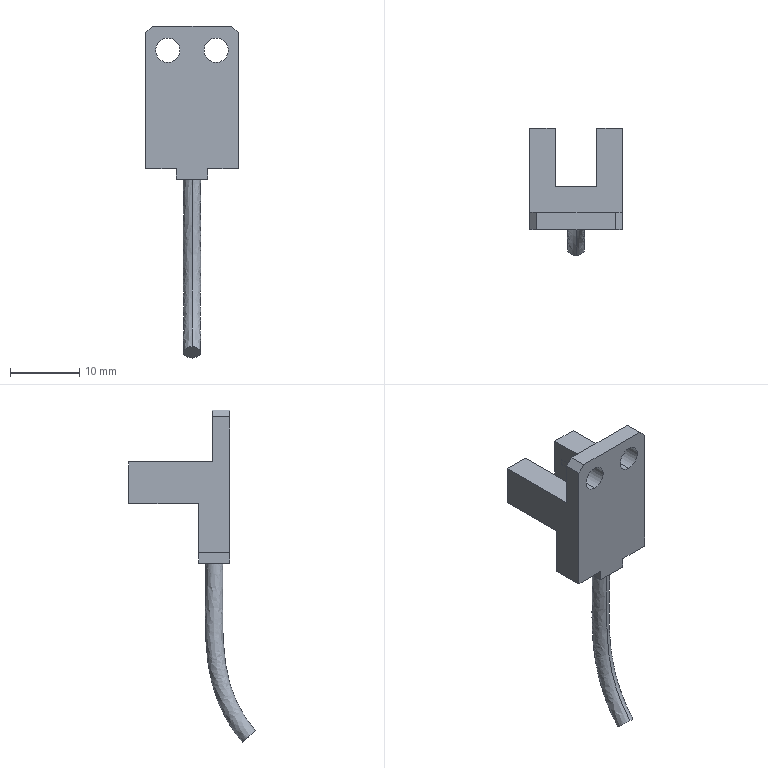Part | NX | features BREP 1 | 1 solid | 41 faces | box 13.4 x 18.3 x 47.912 mm | volume 1659 mm3 | plane 33 | cylinder 6 | spline 2 | commonest cylinder face diameters 3.5 x4 1 x2
STEP:
#1=CARTESIAN_POINT('',(1.25,2.25,-8.6));
#2=VERTEX_POINT('',#1);
#3=CARTESIAN_POINT('',(0.,0.9995,-8.6));
#4=VERTEX_POINT('',#3);
#5=CARTESIAN_POINT('',(1.25,2.25,-8.6));
#6=CARTESIAN_POINT('',(1.25,1.59,-8.6));
#7=CARTESIAN_POINT('',(0.6604,0.9995,-8.6));
#8=CARTESIAN_POINT('',(0.,0.9995,-8.6));
#9=B_SPLINE_CURVE_WITH_KNOTS('',3,(#5,#6,#7,#8),.UNSPECIFIED.,.F.,.F.,(4,4),(0.,0.001953),.UNSPECIFIED.);
#10=EDGE_CURVE('',#2,#4,#9,.T.);
#11=ORIENTED_EDGE('',*,*,#10,.T.);
#12=CARTESIAN_POINT('',(0.,-3.7,-32.788));
#13=VERTEX_POINT('',#12);
#14=CARTESIAN_POINT('',(0.,0.9995,-8.6));
#15=CARTESIAN_POINT('',(0.,0.8731,-12.965));
#16=CARTESIAN_POINT('',(0.,1.227,-17.286));
#17=CARTESIAN_POINT('',(0.,0.4346,-25.439));
#18=CARTESIAN_POINT('',(0.,-0.6656,-29.235));
#19=CARTESIAN_POINT('',(0.,-3.7,-32.788));
#20=B_SPLINE_CURVE_WITH_KNOTS('',3,(#14,#15,#16,#17,#18,#19),.UNSPECIFIED.,.F.,.F.,(4,2,4),(0.,0.4993,1.),.UNSPECIFIED.);
#21=EDGE_CURVE('',#4,#13,#20,.T.);
#22=ORIENTED_EDGE('',*,*,#21,.T.);
#23=CARTESIAN_POINT('',(0.,-1.8,-34.412));
#24=VERTEX_POINT('',#23);
#25=CARTESIAN_POINT('',(0.,-2.75,-33.6));
#26=DIRECTION('',(0.,-0.6495,-0.7604));
#27=DIRECTION('',(0.,0.7604,-0.6495));
#28=AXIS2_PLACEMENT_3D('',#25,#26,#27);
#29=CIRCLE('',#28,1.25);
#30=EDGE_CURVE('',#24,#13,#29,.T.);
#31=ORIENTED_EDGE('',*,*,#30,.F.);
#32=CARTESIAN_POINT('',(0.,3.499,-8.637));
#33=VERTEX_POINT('',#32);
#34=CARTESIAN_POINT('',(0.,3.499,-8.637));
#35=CARTESIAN_POINT('',(0.,3.376,-12.823));
#36=CARTESIAN_POINT('',(0.,3.746,-17.21));
#37=CARTESIAN_POINT('',(0.,2.893,-25.986));
#38=CARTESIAN_POINT('',(0.,1.62,-30.408));
#39=CARTESIAN_POINT('',(0.,-1.8,-34.412));
#40=B_SPLINE_CURVE_WITH_KNOTS('',3,(#34,#35,#36,#37,#38,#39),.UNSPECIFIED.,.F.,.F.,(4,2,4),(0.,0.5,1.),.UNSPECIFIED.);
#41=EDGE_CURVE('',#33,#24,#40,.T.);
#42=ORIENTED_EDGE('',*,*,#41,.F.);
#43=CARTESIAN_POINT('',(0.,2.25,-8.6));
#44=DIRECTION('',(0.,-0.02956,-0.9996));
#45=DIRECTION('',(0.,0.9996,-0.02956));
#46=AXIS2_PLACEMENT_3D('',#43,#44,#45);
#47=CIRCLE('',#46,1.25);
#48=EDGE_CURVE('',#33,#2,#47,.T.);
#49=ORIENTED_EDGE('',*,*,#48,.T.);
#50=EDGE_LOOP('',(#11,#22,#31,#42,#49));
#51=FACE_BOUND('',#50,.T.);
#52=CARTESIAN_POINT('',(0.,3.499,-8.637));
#53=CARTESIAN_POINT('',(0.,3.376,-12.823));
#54=CARTESIAN_POINT('',(0.,3.746,-17.21));
#55=CARTESIAN_POINT('',(0.,2.893,-25.986));
#56=CARTESIAN_POINT('',(0.,1.62,-30.408));
#57=CARTESIAN_POINT('',(0.,-1.8,-34.412));
#58=CARTESIAN_POINT('',(2.5,3.499,-8.637));
#59=CARTESIAN_POINT('',(2.5,3.376,-12.823));
#60=CARTESIAN_POINT('',(2.5,3.746,-17.21));
#61=CARTESIAN_POINT('',(2.5,2.893,-25.986));
#62=CARTESIAN_POINT('',(2.5,1.62,-30.408));
#63=CARTESIAN_POINT('',(2.5,-1.8,-34.412));
#64=CARTESIAN_POINT('',(2.5,1.001,-8.563));
#65=CARTESIAN_POINT('',(2.5,0.8711,-12.94));
#66=CARTESIAN_POINT('',(2.5,1.228,-17.274));
#67=CARTESIAN_POINT('',(2.5,0.4346,-25.439));
#68=CARTESIAN_POINT('',(2.5,-0.6656,-29.235));
#69=CARTESIAN_POINT('',(2.5,-3.7,-32.788));
#70=CARTESIAN_POINT('',(0.,1.001,-8.563));
#71=CARTESIAN_POINT('',(0.,0.8711,-12.94));
#72=CARTESIAN_POINT('',(0.,1.228,-17.274));
#73=CARTESIAN_POINT('',(0.,0.4346,-25.439));
#74=CARTESIAN_POINT('',(0.,-0.6656,-29.235));
#75=CARTESIAN_POINT('',(0.,-3.7,-32.788));
#76=(BOUNDED_SURFACE()B_SPLINE_SURFACE(3,3,((#52,#53,#54,#55,#56,#57),(#58,#59,#60,#61,#62,#63),(#64,#65,#66,#67,#68,#69),(#70,#71,#72,#73,#74,#75)),.UNSPECIFIED.,.F.,.F.,.F.)B_SPLINE_SURFACE_WITH_KNOTS((4,4),(4,2,4),(0.,0.5),(0.,0.5,1.),.UNSPECIFIED.)GEOMETRIC_REPRESENTATION_ITEM()RATIONAL_B_SPLINE_SURFACE(((1.,1.,1.,1.,1.,1.),(0.3333,0.3333,0.3333,0.3333,0.3333,0.3333),(0.3333,0.3333,0.3333,0.3333,0.3333,0.3333),(1.,1.,1.,1.,1.,1.)))REPRESENTATION_ITEM('')SURFACE());
#77=ADVANCED_FACE('',(#51),#76,.T.);
#78=CARTESIAN_POINT('',(3.502,2.5,11.75));
#79=VERTEX_POINT('',#78);
#80=CARTESIAN_POINT('',(3.502,2.5,8.25));
#81=VERTEX_POINT('',#80);
#82=CARTESIAN_POINT('',(3.502,2.5,10.));
#83=DIRECTION('',(0.,-1.,0.));
#84=DIRECTION('',(0.,0.,-1.));
#85=AXIS2_PLACEMENT_3D('',#82,#83,#84);
#86=CIRCLE('',#85,1.75);
#87=EDGE_CURVE('',#79,#81,#86,.T.);
#88=ORIENTED_EDGE('',*,*,#87,.F.);
#89=CARTESIAN_POINT('',(3.502,0.,11.75));
#90=VERTEX_POINT('',#89);
#91=CARTESIAN_POINT('',(3.502,14.6,11.75));
#92=DIRECTION('',(0.,-1.,0.));
#93=VECTOR('',#92,1000.);
#94=LINE('',#91,#93);
#95=EDGE_CURVE('',#90,#79,#94,.F.);
#96=ORIENTED_EDGE('',*,*,#95,.F.);
#97=CARTESIAN_POINT('',(3.502,0.,8.25));
#98=VERTEX_POINT('',#97);
#99=CARTESIAN_POINT('',(3.502,0.,10.));
#100=DIRECTION('',(0.,1.,0.));
#101=DIRECTION('',(0.,0.,1.));
#102=AXIS2_PLACEMENT_3D('',#99,#100,#101);
#103=CIRCLE('',#102,1.75);
#104=EDGE_CURVE('',#98,#90,#103,.T.);
#105=ORIENTED_EDGE('',*,*,#104,.F.);
#106=CARTESIAN_POINT('',(3.502,14.6,8.25));
#107=DIRECTION('',(0.,-1.,0.));
#108=VECTOR('',#107,1000.);
#109=LINE('',#106,#108);
#110=EDGE_CURVE('',#98,#81,#109,.F.);
#111=ORIENTED_EDGE('',*,*,#110,.T.);
#112=EDGE_LOOP('',(#88,#96,#105,#111));
#113=FACE_BOUND('',#112,.T.);
#114=CARTESIAN_POINT('',(3.502,14.6,10.));
#115=DIRECTION('',(0.,-1.,0.));
#116=DIRECTION('',(0.,0.,1.));
#117=AXIS2_PLACEMENT_3D('',#114,#115,#116);
#118=CYLINDRICAL_SURFACE('',#117,1.75);
#119=ADVANCED_FACE('',(#113),#118,.F.);
#120=CARTESIAN_POINT('',(-3.502,2.5,11.75));
#121=VERTEX_POINT('',#120);
#122=CARTESIAN_POINT('',(-3.502,2.5,8.25));
#123=VERTEX_POINT('',#122);
#124=CARTESIAN_POINT('',(-3.502,2.5,10.));
#125=DIRECTION('',(0.,-1.,0.));
#126=DIRECTION('',(0.,0.,-1.));
#127=AXIS2_PLACEMENT_3D('',#124,#125,#126);
#128=CIRCLE('',#127,1.75);
#129=EDGE_CURVE('',#121,#123,#128,.T.);
#130=ORIENTED_EDGE('',*,*,#129,.F.);
#131=CARTESIAN_POINT('',(-3.502,0.,11.75));
#132=VERTEX_POINT('',#131);
#133=CARTESIAN_POINT('',(-3.502,14.6,11.75));
#134=DIRECTION('',(0.,-1.,0.));
#135=VECTOR('',#134,1000.);
#136=LINE('',#133,#135);
#137=EDGE_CURVE('',#132,#121,#136,.F.);
#138=ORIENTED_EDGE('',*,*,#137,.F.);
#139=CARTESIAN_POINT('',(-3.502,0.,8.25));
#140=VERTEX_POINT('',#139);
#141=CARTESIAN_POINT('',(-3.502,0.,10.));
#142=DIRECTION('',(0.,1.,0.));
#143=DIRECTION('',(0.,0.,1.));
#144=AXIS2_PLACEMENT_3D('',#141,#142,#143);
#145=CIRCLE('',#144,1.75);
#146=EDGE_CURVE('',#140,#132,#145,.T.);
#147=ORIENTED_EDGE('',*,*,#146,.F.);
#148=CARTESIAN_POINT('',(-3.502,14.6,8.25));
#149=DIRECTION('',(0.,-1.,0.));
#150=VECTOR('',#149,1000.);
#151=LINE('',#148,#150);
#152=EDGE_CURVE('',#140,#123,#151,.F.);
#153=ORIENTED_EDGE('',*,*,#152,.T.);
#154=EDGE_LOOP('',(#130,#138,#147,#153));
#155=FACE_BOUND('',#154,.T.);
#156=CARTESIAN_POINT('',(-3.502,14.6,10.));
#157=DIRECTION('',(0.,-1.,0.));
#158=DIRECTION('',(0.,0.,1.));
#159=AXIS2_PLACEMENT_3D('',#156,#157,#158);
#160=CYLINDRICAL_SURFACE('',#159,1.75);
#161=ADVANCED_FACE('',(#155),#160,.F.);
#162=CARTESIAN_POINT('',(0.,6.21,3.5));
#163=VERTEX_POINT('',#162);
#164=CARTESIAN_POINT('',(0.,6.21,2.5));
#165=VERTEX_POINT('',#164);
#166=CARTESIAN_POINT('',(0.,6.21,3.));
#167=DIRECTION('',(0.,1.,0.));
#168=DIRECTION('',(0.,0.,1.));
#169=AXIS2_PLACEMENT_3D('',#166,#167,#168);
#170=CIRCLE('',#169,0.5);
#171=EDGE_CURVE('',#163,#165,#170,.T.);
#172=ORIENTED_EDGE('',*,*,#171,.F.);
#173=CARTESIAN_POINT('',(0.,6.2,3.5));
#174=VERTEX_POINT('',#173);
#175=CARTESIAN_POINT('',(0.,6.21,3.5));
#176=DIRECTION('',(0.,-1.,0.));
#177=VECTOR('',#176,1000.);
#178=LINE('',#175,#177);
#179=EDGE_CURVE('',#174,#163,#178,.F.);
#180=ORIENTED_EDGE('',*,*,#179,.F.);
#181=CARTESIAN_POINT('',(0.,6.2,2.5));
#182=VERTEX_POINT('',#181);
#183=CARTESIAN_POINT('',(0.,6.2,3.));
#184=DIRECTION('',(0.,1.,0.));
#185=DIRECTION('',(0.,0.,-1.));
#186=AXIS2_PLACEMENT_3D('',#183,#184,#185);
#187=CIRCLE('',#186,0.5);
#188=EDGE_CURVE('',#174,#182,#187,.T.);
#189=ORIENTED_EDGE('',*,*,#188,.T.);
#190=CARTESIAN_POINT('',(0.,6.21,2.5));
#191=DIRECTION('',(0.,-1.,0.));
#192=VECTOR('',#191,1000.);
#193=LINE('',#190,#192);
#194=EDGE_CURVE('',#182,#165,#193,.F.);
#195=ORIENTED_EDGE('',*,*,#194,.T.);
#196=EDGE_LOOP('',(#172,#180,#189,#195));
#197=FACE_BOUND('',#196,.T.);
#198=CARTESIAN_POINT('',(0.,6.21,3.));
#199=DIRECTION('',(0.,-1.,0.));
#200=DIRECTION('',(0.,0.,1.));
#201=AXIS2_PLACEMENT_3D('',#198,#199,#200);
#202=CYLINDRICAL_SURFACE('',#201,0.5);
#203=ADVANCED_FACE('',(#197),#202,.T.);
#204=CARTESIAN_POINT('',(2.25,4.5,-8.6));
#205=VERTEX_POINT('',#204);
#206=CARTESIAN_POINT('',(2.25,0.,-8.6));
#207=VERTEX_POINT('',#206);
#208=CARTESIAN_POINT('',(2.25,4.5,-8.6));
#209=DIRECTION('',(0.,-1.,0.));
#210=VECTOR('',#209,1000.);
#211=LINE('',#208,#210);
#212=EDGE_CURVE('',#205,#207,#211,.T.);
#213=ORIENTED_EDGE('',*,*,#212,.T.);
#214=CARTESIAN_POINT('',(-2.25,0.,-8.6));
#215=VERTEX_POINT('',#214);
#216=CARTESIAN_POINT('',(2.25,0.,-8.6));
#217=DIRECTION('',(-1.,0.,0.));
#218=VECTOR('',#217,1000.);
#219=LINE('',#216,#218);
#220=EDGE_CURVE('',#207,#215,#219,.T.);
#221=ORIENTED_EDGE('',*,*,#220,.T.);
#222=CARTESIAN_POINT('',(-2.25,4.5,-8.6));
#223=VERTEX_POINT('',#222);
#224=CARTESIAN_POINT('',(-2.25,4.5,-8.6));
#225=DIRECTION('',(0.,1.,0.));
#226=VECTOR('',#225,1000.);
#227=LINE('',#224,#226);
#228=EDGE_CURVE('',#215,#223,#227,.T.);
#229=ORIENTED_EDGE('',*,*,#228,.T.);
#230=CARTESIAN_POINT('',(2.25,4.5,-8.6));
#231=DIRECTION('',(1.,0.,0.));
#232=VECTOR('',#231,1000.);
#233=LINE('',#230,#232);
#234=EDGE_CURVE('',#223,#205,#233,.T.);
#235=ORIENTED_EDGE('',*,*,#234,.T.);
#236=EDGE_LOOP('',(#213,#221,#229,#235));
#237=FACE_BOUND('',#236,.T.);
#238=ORIENTED_EDGE('',*,*,#10,.F.);
#239=CARTESIAN_POINT('',(-1.25,2.25,-8.6));
#240=VERTEX_POINT('',#239);
#241=CARTESIAN_POINT('',(0.,2.25,-8.6));
#242=DIRECTION('',(-1.,0.,0.));
#243=VECTOR('',#242,1000.);
#244=LINE('',#241,#243);
#245=EDGE_CURVE('',#2,#240,#244,.T.);
#246=ORIENTED_EDGE('',*,*,#245,.T.);
#247=CARTESIAN_POINT('',(0.,0.9995,-8.6));
#248=CARTESIAN_POINT('',(-0.6604,0.9995,-8.6));
#249=CARTESIAN_POINT('',(-1.25,1.59,-8.6));
#250=CARTESIAN_POINT('',(-1.25,2.25,-8.6));
#251=B_SPLINE_CURVE_WITH_KNOTS('',3,(#247,#248,#249,#250),.UNSPECIFIED.,.F.,.F.,(4,4),(0.,0.001953),.UNSPECIFIED.);
#252=EDGE_CURVE('',#4,#240,#251,.T.);
#253=ORIENTED_EDGE('',*,*,#252,.F.);
#254=EDGE_LOOP('',(#238,#246,#253));
#255=FACE_BOUND('',#254,.T.);
#256=CARTESIAN_POINT('',(0.,0.,-8.6));
#257=DIRECTION('',(0.,0.,-1.));
#258=DIRECTION('',(1.,0.,0.));
#259=AXIS2_PLACEMENT_3D('',#256,#257,#258);
#260=PLANE('',#259);
#261=ADVANCED_FACE('',(#237,#255),#260,.T.);
#262=CARTESIAN_POINT('',(2.25,4.5,-7.1));
#263=VERTEX_POINT('',#262);
#264=CARTESIAN_POINT('',(2.25,0.,-7.1));
#265=VERTEX_POINT('',#264);
#266=CARTESIAN_POINT('',(2.25,4.5,-7.1));
#267=DIRECTION('',(0.,-1.,0.));
#268=VECTOR('',#267,1000.);
#269=LINE('',#266,#268);
#270=EDGE_CURVE('',#263,#265,#269,.T.);
#271=ORIENTED_EDGE('',*,*,#270,.F.);
#272=CARTESIAN_POINT('',(6.7,4.5,-7.1));
#273=VERTEX_POINT('',#272);
#274=CARTESIAN_POINT('',(-6.7,4.5,-7.1));
#275=DIRECTION('',(1.,0.,0.));
#276=VECTOR('',#275,1000.);
#277=LINE('',#274,#276);
#278=EDGE_CURVE('',#263,#273,#277,.T.);
#279=ORIENTED_EDGE('',*,*,#278,.T.);
#280=CARTESIAN_POINT('',(6.7,0.,-7.1));
#281=VERTEX_POINT('',#280);
#282=CARTESIAN_POINT('',(6.7,4.5,-7.1));
#283=DIRECTION('',(0.,-1.,0.));
#284=VECTOR('',#283,1000.);
#285=LINE('',#282,#284);
#286=EDGE_CURVE('',#273,#281,#285,.T.);
#287=ORIENTED_EDGE('',*,*,#286,.T.);
#288=CARTESIAN_POINT('',(-6.7,0.,-7.1));
#289=DIRECTION('',(1.,0.,0.));
#290=VECTOR('',#289,1000.);
#291=LINE('',#288,#290);
#292=EDGE_CURVE('',#265,#281,#291,.T.);
#293=ORIENTED_EDGE('',*,*,#292,.F.);
#294=EDGE_LOOP('',(#271,#279,#287,#293));
#295=FACE_BOUND('',#294,.T.);
#296=CARTESIAN_POINT('',(-6.7,4.5,-7.1));
#297=DIRECTION('',(0.,0.,-1.));
#298=DIRECTION('',(1.,0.,0.));
#299=AXIS2_PLACEMENT_3D('',#296,#297,#298);
#300=PLANE('',#299);
#301=ADVANCED_FACE('',(#295),#300,.T.);
#302=CARTESIAN_POINT('',(6.7,4.5,0.));
#303=VERTEX_POINT('',#302);
#304=CARTESIAN_POINT('',(6.7,14.6,0.));
#305=VERTEX_POINT('',#304);
#306=CARTESIAN_POINT('',(6.7,14.6,0.));
#307=DIRECTION('',(0.,1.,0.));
#308=VECTOR('',#307,1000.);
#309=LINE('',#306,#308);
#310=EDGE_CURVE('',#303,#305,#309,.T.);
#311=ORIENTED_EDGE('',*,*,#310,.F.);
#312=CARTESIAN_POINT('',(-6.7,4.5,0.));
#313=VERTEX_POINT('',#312);
#314=CARTESIAN_POINT('',(-6.7,4.5,0.));
#315=DIRECTION('',(-1.,0.,0.));
#316=VECTOR('',#315,1000.);
#317=LINE('',#314,#316);
#318=EDGE_CURVE('',#303,#313,#317,.T.);
#319=ORIENTED_EDGE('',*,*,#318,.T.);
#320=CARTESIAN_POINT('',(-6.7,14.6,0.));
#321=VERTEX_POINT('',#320);
#322=CARTESIAN_POINT('',(-6.7,14.6,0.));
#323=DIRECTION('',(0.,-1.,0.));
#324=VECTOR('',#323,1000.);
#325=LINE('',#322,#324);
#326=EDGE_CURVE('',#321,#313,#325,.T.);
#327=ORIENTED_EDGE('',*,*,#326,.F.);
#328=CARTESIAN_POINT('',(-3.,14.6,0.));
#329=VERTEX_POINT('',#328);
#330=CARTESIAN_POINT('',(-3.,14.6,0.));
#331=DIRECTION('',(-1.,0.,0.));
#332=VECTOR('',#331,1000.);
#333=LINE('',#330,#332);
#334=EDGE_CURVE('',#329,#321,#333,.T.);
#335=ORIENTED_EDGE('',*,*,#334,.F.);
#336=CARTESIAN_POINT('',(-3.,6.2,0.));
#337=VERTEX_POINT('',#336);
#338=CARTESIAN_POINT('',(-3.,6.2,0.));
#339=DIRECTION('',(0.,1.,0.));
#340=VECTOR('',#339,1000.);
#341=LINE('',#338,#340);
#342=EDGE_CURVE('',#337,#329,#341,.T.);
#343=ORIENTED_EDGE('',*,*,#342,.F.);
#344=CARTESIAN_POINT('',(3.,6.2,0.));
#345=VERTEX_POINT('',#344);
#346=CARTESIAN_POINT('',(3.,6.2,0.));
#347=DIRECTION('',(-1.,0.,0.));
#348=VECTOR('',#347,1000.);
#349=LINE('',#346,#348);
#350=EDGE_CURVE('',#345,#337,#349,.T.);
#351=ORIENTED_EDGE('',*,*,#350,.F.);
#352=CARTESIAN_POINT('',(3.,14.6,0.));
#353=VERTEX_POINT('',#352);
#354=CARTESIAN_POINT('',(3.,6.2,0.));
#355=DIRECTION('',(0.,-1.,0.));
#356=VECTOR('',#355,1000.);
#357=LINE('',#354,#356);
#358=EDGE_CURVE('',#353,#345,#357,.T.);
#359=ORIENTED_EDGE('',*,*,#358,.F.);
#360=CARTESIAN_POINT('',(3.,14.6,0.));
#361=DIRECTION('',(-1.,0.,0.));
#362=VECTOR('',#361,1000.);
#363=LINE('',#360,#362);
#364=EDGE_CURVE('',#305,#353,#363,.T.);
#365=ORIENTED_EDGE('',*,*,#364,.F.);
#366=EDGE_LOOP('',(#311,#319,#327,#335,#343,#351,#359,#365));
#367=FACE_BOUND('',#366,.T.);
#368=CARTESIAN_POINT('',(0.,0.,0.));
#369=DIRECTION('',(0.,0.,-1.));
#370=DIRECTION('',(1.,0.,0.));
#371=AXIS2_PLACEMENT_3D('',#368,#369,#370);
#372=PLANE('',#371);
#373=ADVANCED_FACE('',(#367),#372,.T.);
#374=ORIENTED_EDGE('',*,*,#342,.T.);
#375=CARTESIAN_POINT('',(-3.,14.6,6.));
#376=VERTEX_POINT('',#375);
#377=CARTESIAN_POINT('',(-3.,14.6,6.));
#378=DIRECTION('',(0.,0.,-1.));
#379=VECTOR('',#378,1000.);
#380=LINE('',#377,#379);
#381=EDGE_CURVE('',#376,#329,#380,.T.);
#382=ORIENTED_EDGE('',*,*,#381,.F.);
#383=CARTESIAN_POINT('',(-3.,6.2,6.));
#384=VERTEX_POINT('',#383);
#385=CARTESIAN_POINT('',(-3.,6.2,6.));
#386=DIRECTION('',(0.,1.,0.));
#387=VECTOR('',#386,1000.);
#388=LINE('',#385,#387);
#389=EDGE_CURVE('',#384,#376,#388,.T.);
#390=ORIENTED_EDGE('',*,*,#389,.F.);
#391=CARTESIAN_POINT('',(-3.,6.2,6.));
#392=DIRECTION('',(0.,0.,-1.));
#393=VECTOR('',#392,1000.);
#394=LINE('',#391,#393);
#395=EDGE_CURVE('',#384,#337,#394,.T.);
#396=ORIENTED_EDGE('',*,*,#395,.T.);
#397=EDGE_LOOP('',(#374,#382,#390,#396));
#398=FACE_BOUND('',#397,.T.);
#399=CARTESIAN_POINT('',(-3.,12.,2.6));
#400=VERTEX_POINT('',#399);
#401=CARTESIAN_POINT('',(-3.,13.2,2.6));
#402=VERTEX_POINT('',#401);
#403=CARTESIAN_POINT('',(-3.,13.2,2.6));
#404=DIRECTION('',(0.,1.,0.));
#405=VECTOR('',#404,1000.);
#406=LINE('',#403,#405);
#407=EDGE_CURVE('',#400,#402,#406,.T.);
#408=ORIENTED_EDGE('',*,*,#407,.F.);
#409=CARTESIAN_POINT('',(-3.,12.,3.4));
#410=VERTEX_POINT('',#409);
#411=CARTESIAN_POINT('',(-3.,12.,3.4));
#412=DIRECTION('',(0.,0.,-1.));
#413=VECTOR('',#412,1000.);
#414=LINE('',#411,#413);
#415=EDGE_CURVE('',#410,#400,#414,.T.);
#416=ORIENTED_EDGE('',*,*,#415,.F.);
#417=CARTESIAN_POINT('',(-3.,13.2,3.4));
#418=VERTEX_POINT('',#417);
#419=CARTESIAN_POINT('',(-3.,13.2,3.4));
#420=DIRECTION('',(0.,-1.,0.));
#421=VECTOR('',#420,1000.);
#422=LINE('',#419,#421);
#423=EDGE_CURVE('',#418,#410,#422,.T.);
#424=ORIENTED_EDGE('',*,*,#423,.F.);
#425=CARTESIAN_POINT('',(-3.,13.2,3.4));
#426=DIRECTION('',(0.,0.,1.));
#427=VECTOR('',#426,1000.);
#428=LINE('',#425,#427);
#429=EDGE_CURVE('',#402,#418,#428,.T.);
#430=ORIENTED_EDGE('',*,*,#429,.F.);
#431=EDGE_LOOP('',(#408,#416,#424,#430));
#432=FACE_BOUND('',#431,.T.);
#433=CARTESIAN_POINT('',(-3.,6.2,6.));
#434=DIRECTION('',(-1.,0.,0.));
#435=DIRECTION('',(0.,0.,-1.));
#436=AXIS2_PLACEMENT_3D('',#433,#434,#435);
#437=PLANE('',#436);
#438=ADVANCED_FACE('',(#398,#432),#437,.F.);
#439=CARTESIAN_POINT('',(0.,6.2,3.));
#440=DIRECTION('',(0.,1.,0.));
#441=DIRECTION('',(0.,0.,-1.));
#442=AXIS2_PLACEMENT_3D('',#439,#440,#441);
#443=CIRCLE('',#442,0.5);
#444=EDGE_CURVE('',#182,#174,#443,.T.);
#445=ORIENTED_EDGE('',*,*,#444,.F.);
#446=ORIENTED_EDGE('',*,*,#188,.F.);
#447=EDGE_LOOP('',(#445,#446));
#448=FACE_BOUND('',#447,.T.);
#449=ORIENTED_EDGE('',*,*,#350,.T.);
#450=ORIENTED_EDGE('',*,*,#395,.F.);
#451=CARTESIAN_POINT('',(3.,6.2,6.));
#452=VERTEX_POINT('',#451);
#453=CARTESIAN_POINT('',(3.,6.2,6.));
#454=DIRECTION('',(-1.,0.,0.));
#455=VECTOR('',#454,1000.);
#456=LINE('',#453,#455);
#457=EDGE_CURVE('',#452,#384,#456,.T.);
#458=ORIENTED_EDGE('',*,*,#457,.F.);
#459=CARTESIAN_POINT('',(3.,6.2,6.));
#460=DIRECTION('',(0.,0.,-1.));
#461=VECTOR('',#460,1000.);
#462=LINE('',#459,#461);
#463=EDGE_CURVE('',#452,#345,#462,.T.);
#464=ORIENTED_EDGE('',*,*,#463,.T.);
#465=EDGE_LOOP('',(#449,#450,#458,#464));
#466=FACE_BOUND('',#465,.T.);
#467=CARTESIAN_POINT('',(3.,6.2,6.));
#468=DIRECTION('',(0.,-1.,0.));
#469=DIRECTION('',(0.,0.,1.));
#470=AXIS2_PLACEMENT_3D('',#467,#468,#469);
#471=PLANE('',#470);
#472=ADVANCED_FACE('',(#448,#466),#471,.F.);
#473=ORIENTED_EDGE('',*,*,#334,.T.);
#474=CARTESIAN_POINT('',(-6.7,14.6,6.));
#475=VERTEX_POINT('',#474);
#476=CARTESIAN_POINT('',(-6.7,14.6,6.));
#477=DIRECTION('',(0.,0.,-1.));
#478=VECTOR('',#477,1000.);
#479=LINE('',#476,#478);
#480=EDGE_CURVE('',#475,#321,#479,.T.);
#481=ORIENTED_EDGE('',*,*,#480,.F.);
#482=CARTESIAN_POINT('',(-3.,14.6,6.));
#483=DIRECTION('',(-1.,0.,0.));
#484=VECTOR('',#483,1000.);
#485=LINE('',#482,#484);
#486=EDGE_CURVE('',#376,#475,#485,.T.);
#487=ORIENTED_EDGE('',*,*,#486,.F.);
#488=ORIENTED_EDGE('',*,*,#381,.T.);
#489=EDGE_LOOP('',(#473,#481,#487,#488));
#490=FACE_BOUND('',#489,.T.);
#491=CARTESIAN_POINT('',(-3.,14.6,6.));
#492=DIRECTION('',(0.,-1.,0.));
#493=DIRECTION('',(0.,0.,1.));
#494=AXIS2_PLACEMENT_3D('',#491,#492,#493);
#495=PLANE('',#494);
#496=ADVANCED_FACE('',(#490),#495,.F.);
#497=CARTESIAN_POINT('',(-6.7,0.,12.5));
#498=VERTEX_POINT('',#497);
#499=CARTESIAN_POINT('',(-6.7,0.,-7.1));
#500=VERTEX_POINT('',#499);
#501=CARTESIAN_POINT('',(-6.7,0.,6.));
#502=DIRECTION('',(0.,0.,-1.));
#503=VECTOR('',#502,1000.);
#504=LINE('',#501,#503);
#505=EDGE_CURVE('',#498,#500,#504,.T.);
#506=ORIENTED_EDGE('',*,*,#505,.F.);
#507=CARTESIAN_POINT('',(-6.7,2.5,12.5));
#508=VERTEX_POINT('',#507);
#509=CARTESIAN_POINT('',(-6.7,2.5,12.5));
#510=DIRECTION('',(0.,1.,0.));
#511=VECTOR('',#510,1000.);
#512=LINE('',#509,#511);
#513=EDGE_CURVE('',#498,#508,#512,.T.);
#514=ORIENTED_EDGE('',*,*,#513,.T.);
#515=CARTESIAN_POINT('',(-6.7,2.5,6.));
#516=VERTEX_POINT('',#515);
#517=CARTESIAN_POINT('',(-6.7,2.5,13.5));
#518=DIRECTION('',(0.,0.,-1.));
#519=VECTOR('',#518,1000.);
#520=LINE('',#517,#519);
#521=EDGE_CURVE('',#508,#516,#520,.T.);
#522=ORIENTED_EDGE('',*,*,#521,.T.);
#523=CARTESIAN_POINT('',(-6.7,14.6,6.));
#524=DIRECTION('',(0.,-1.,0.));
#525=VECTOR('',#524,1000.);
#526=LINE('',#523,#525);
#527=EDGE_CURVE('',#475,#516,#526,.T.);
#528=ORIENTED_EDGE('',*,*,#527,.F.);
#529=ORIENTED_EDGE('',*,*,#480,.T.);
#530=ORIENTED_EDGE('',*,*,#326,.T.);
#531=CARTESIAN_POINT('',(-6.7,4.5,-7.1));
#532=VERTEX_POINT('',#531);
#533=CARTESIAN_POINT('',(-6.7,4.5,0.));
#534=DIRECTION('',(0.,0.,-1.));
#535=VECTOR('',#534,1000.);
#536=LINE('',#533,#535);
#537=EDGE_CURVE('',#313,#532,#536,.T.);
#538=ORIENTED_EDGE('',*,*,#537,.T.);
#539=CARTESIAN_POINT('',(-6.7,4.5,-7.1));
#540=DIRECTION('',(0.,-1.,0.));
#541=VECTOR('',#540,1000.);
#542=LINE('',#539,#541);
#543=EDGE_CURVE('',#532,#500,#542,.T.);
#544=ORIENTED_EDGE('',*,*,#543,.T.);
#545=EDGE_LOOP('',(#506,#514,#522,#528,#529,#530,#538,#544));
#546=FACE_BOUND('',#545,.T.);
#547=CARTESIAN_POINT('',(-6.7,14.6,6.));
#548=DIRECTION('',(1.,0.,0.));
#549=DIRECTION('',(0.,-1.,0.));
#550=AXIS2_PLACEMENT_3D('',#547,#548,#549);
#551=PLANE('',#550);
#552=ADVANCED_FACE('',(#546),#551,.F.);
#553=ORIENTED_EDGE('',*,*,#104,.T.);
#554=CARTESIAN_POINT('',(3.502,0.,10.));
#555=DIRECTION('',(0.,1.,0.));
#556=DIRECTION('',(0.,0.,1.));
#557=AXIS2_PLACEMENT_3D('',#554,#555,#556);
#558=CIRCLE('',#557,1.75);
#559=EDGE_CURVE('',#90,#98,#558,.T.);
#560=ORIENTED_EDGE('',*,*,#559,.T.);
#561=EDGE_LOOP('',(#553,#560));
#562=FACE_BOUND('',#561,.T.);
#563=ORIENTED_EDGE('',*,*,#146,.T.);
#564=CARTESIAN_POINT('',(-3.502,0.,10.));
#565=DIRECTION('',(0.,1.,0.));
#566=DIRECTION('',(0.,0.,1.));
#567=AXIS2_PLACEMENT_3D('',#564,#565,#566);
#568=CIRCLE('',#567,1.75);
#569=EDGE_CURVE('',#132,#140,#568,.T.);
#570=ORIENTED_EDGE('',*,*,#569,.T.);
#571=EDGE_LOOP('',(#563,#570));
#572=FACE_BOUND('',#571,.T.);
#573=CARTESIAN_POINT('',(6.7,0.,12.5));
#574=VERTEX_POINT('',#573);
#575=CARTESIAN_POINT('',(6.7,0.,6.));
#576=DIRECTION('',(0.,0.,-1.));
#577=VECTOR('',#576,1000.);
#578=LINE('',#575,#577);
#579=EDGE_CURVE('',#574,#281,#578,.T.);
#580=ORIENTED_EDGE('',*,*,#579,.F.);
#581=CARTESIAN_POINT('',(5.7,0.,13.5));
#582=VERTEX_POINT('',#581);
#583=CARTESIAN_POINT('',(6.7,0.,12.5));
#584=DIRECTION('',(-0.7071,0.,0.7071));
#585=VECTOR('',#584,1000.);
#586=LINE('',#583,#585);
#587=EDGE_CURVE('',#574,#582,#586,.T.);
#588=ORIENTED_EDGE('',*,*,#587,.T.);
#589=CARTESIAN_POINT('',(-5.7,0.,13.5));
#590=VERTEX_POINT('',#589);
#591=CARTESIAN_POINT('',(-6.7,0.,13.5));
#592=DIRECTION('',(-1.,0.,0.));
#593=VECTOR('',#592,1000.);
#594=LINE('',#591,#593);
#595=EDGE_CURVE('',#582,#590,#594,.T.);
#596=ORIENTED_EDGE('',*,*,#595,.T.);
#597=CARTESIAN_POINT('',(-5.7,0.,13.5));
#598=DIRECTION('',(-0.7071,0.,-0.7071));
#599=VECTOR('',#598,1000.);
#600=LINE('',#597,#599);
#601=EDGE_CURVE('',#590,#498,#600,.T.);
#602=ORIENTED_EDGE('',*,*,#601,.T.);
#603=ORIENTED_EDGE('',*,*,#505,.T.);
#604=CARTESIAN_POINT('',(-2.25,0.,-7.1));
#605=VERTEX_POINT('',#604);
#606=CARTESIAN_POINT('',(-6.7,0.,-7.1));
#607=DIRECTION('',(1.,0.,0.));
#608=VECTOR('',#607,1000.);
#609=LINE('',#606,#608);
#610=EDGE_CURVE('',#500,#605,#609,.T.);
#611=ORIENTED_EDGE('',*,*,#610,.T.);
#612=CARTESIAN_POINT('',(-2.25,0.,-8.6));
#613=DIRECTION('',(0.,0.,1.));
#614=VECTOR('',#613,1000.);
#615=LINE('',#612,#614);
#616=EDGE_CURVE('',#215,#605,#615,.T.);
#617=ORIENTED_EDGE('',*,*,#616,.F.);
#618=ORIENTED_EDGE('',*,*,#220,.F.);
#619=CARTESIAN_POINT('',(2.25,0.,-8.6));
#620=DIRECTION('',(0.,0.,1.));
#621=VECTOR('',#620,1000.);
#622=LINE('',#619,#621);
#623=EDGE_CURVE('',#207,#265,#622,.T.);
#624=ORIENTED_EDGE('',*,*,#623,.T.);
#625=ORIENTED_EDGE('',*,*,#292,.T.);
#626=EDGE_LOOP('',(#580,#588,#596,#602,#603,#611,#617,#618,#624,#625));
#627=FACE_BOUND('',#626,.T.);
#628=CARTESIAN_POINT('',(6.7,0.,6.));
#629=DIRECTION('',(0.,1.,0.));
#630=DIRECTION('',(0.,0.,-1.));
#631=AXIS2_PLACEMENT_3D('',#628,#629,#630);
#632=PLANE('',#631);
#633=ADVANCED_FACE('',(#562,#572,#627),#632,.F.);
#634=CARTESIAN_POINT('',(6.7,2.5,6.));
#635=VERTEX_POINT('',#634);
#636=CARTESIAN_POINT('',(6.7,2.5,12.5));
#637=VERTEX_POINT('',#636);
#638=CARTESIAN_POINT('',(6.7,2.5,13.5));
#639=DIRECTION('',(0.,0.,1.));
#640=VECTOR('',#639,1000.);
#641=LINE('',#638,#640);
#642=EDGE_CURVE('',#635,#637,#641,.T.);
#643=ORIENTED_EDGE('',*,*,#642,.T.);
#644=CARTESIAN_POINT('',(6.7,0.,12.5));
#645=DIRECTION('',(0.,-1.,0.));
#646=VECTOR('',#645,1000.);
#647=LINE('',#644,#646);
#648=EDGE_CURVE('',#637,#574,#647,.T.);
#649=ORIENTED_EDGE('',*,*,#648,.T.);
#650=ORIENTED_EDGE('',*,*,#579,.T.);
#651=ORIENTED_EDGE('',*,*,#286,.F.);
#652=CARTESIAN_POINT('',(6.7,4.5,0.));
#653=DIRECTION('',(0.,0.,1.));
#654=VECTOR('',#653,1000.);
#655=LINE('',#652,#654);
#656=EDGE_CURVE('',#273,#303,#655,.T.);
#657=ORIENTED_EDGE('',*,*,#656,.T.);
#658=ORIENTED_EDGE('',*,*,#310,.T.);
#659=CARTESIAN_POINT('',(6.7,14.6,6.));
#660=VERTEX_POINT('',#659);
#661=CARTESIAN_POINT('',(6.7,14.6,6.));
#662=DIRECTION('',(0.,0.,-1.));
#663=VECTOR('',#662,1000.);
#664=LINE('',#661,#663);
#665=EDGE_CURVE('',#660,#305,#664,.T.);
#666=ORIENTED_EDGE('',*,*,#665,.F.);
#667=CARTESIAN_POINT('',(6.7,14.6,6.));
#668=DIRECTION('',(0.,1.,0.));
#669=VECTOR('',#668,1000.);
#670=LINE('',#667,#669);
#671=EDGE_CURVE('',#635,#660,#670,.T.);
#672=ORIENTED_EDGE('',*,*,#671,.F.);
#673=EDGE_LOOP('',(#643,#649,#650,#651,#657,#658,#666,#672));
#674=FACE_BOUND('',#673,.T.);
#675=CARTESIAN_POINT('',(6.7,14.6,6.));
#676=DIRECTION('',(-1.,0.,0.));
#677=DIRECTION('',(0.,1.,0.));
#678=AXIS2_PLACEMENT_3D('',#675,#676,#677);
#679=PLANE('',#678);
#680=ADVANCED_FACE('',(#674),#679,.F.);
#681=ORIENTED_EDGE('',*,*,#364,.T.);
#682=CARTESIAN_POINT('',(3.,14.6,6.));
#683=VERTEX_POINT('',#682);
#684=CARTESIAN_POINT('',(3.,14.6,6.));
#685=DIRECTION('',(0.,0.,-1.));
#686=VECTOR('',#685,1000.);
#687=LINE('',#684,#686);
#688=EDGE_CURVE('',#683,#353,#687,.T.);
#689=ORIENTED_EDGE('',*,*,#688,.F.);
#690=CARTESIAN_POINT('',(3.,14.6,6.));
#691=DIRECTION('',(-1.,0.,0.));
#692=VECTOR('',#691,1000.);
#693=LINE('',#690,#692);
#694=EDGE_CURVE('',#660,#683,#693,.T.);
#695=ORIENTED_EDGE('',*,*,#694,.F.);
#696=ORIENTED_EDGE('',*,*,#665,.T.);
#697=EDGE_LOOP('',(#681,#689,#695,#696));
#698=FACE_BOUND('',#697,.T.);
#699=CARTESIAN_POINT('',(3.,14.6,6.));
#700=DIRECTION('',(0.,-1.,0.));
#701=DIRECTION('',(0.,0.,1.));
#702=AXIS2_PLACEMENT_3D('',#699,#700,#701);
#703=PLANE('',#702);
#704=ADVANCED_FACE('',(#698),#703,.F.);
#705=CARTESIAN_POINT('',(3.,12.,3.4));
#706=VERTEX_POINT('',#705);
#707=CARTESIAN_POINT('',(3.,12.,2.6));
#708=VERTEX_POINT('',#707);
#709=CARTESIAN_POINT('',(3.,12.,3.4));
#710=DIRECTION('',(0.,0.,-1.));
#711=VECTOR('',#710,1000.);
#712=LINE('',#709,#711);
#713=EDGE_CURVE('',#706,#708,#712,.T.);
#714=ORIENTED_EDGE('',*,*,#713,.T.);
#715=CARTESIAN_POINT('',(3.,13.2,2.6));
#716=VERTEX_POINT('',#715);
#717=CARTESIAN_POINT('',(3.,13.2,2.6));
#718=DIRECTION('',(0.,1.,0.));
#719=VECTOR('',#718,1000.);
#720=LINE('',#717,#719);
#721=EDGE_CURVE('',#708,#716,#720,.T.);
#722=ORIENTED_EDGE('',*,*,#721,.T.);
#723=CARTESIAN_POINT('',(3.,13.2,3.4));
#724=VERTEX_POINT('',#723);
#725=CARTESIAN_POINT('',(3.,13.2,3.4));
#726=DIRECTION('',(0.,0.,1.));
#727=VECTOR('',#726,1000.);
#728=LINE('',#725,#727);
#729=EDGE_CURVE('',#716,#724,#728,.T.);
#730=ORIENTED_EDGE('',*,*,#729,.T.);
#731=CARTESIAN_POINT('',(3.,13.2,3.4));
#732=DIRECTION('',(0.,-1.,0.));
#733=VECTOR('',#732,1000.);
#734=LINE('',#731,#733);
#735=EDGE_CURVE('',#724,#706,#734,.T.);
#736=ORIENTED_EDGE('',*,*,#735,.T.);
#737=EDGE_LOOP('',(#714,#722,#730,#736));
#738=FACE_BOUND('',#737,.T.);
#739=ORIENTED_EDGE('',*,*,#358,.T.);
#740=ORIENTED_EDGE('',*,*,#463,.F.);
#741=CARTESIAN_POINT('',(3.,6.2,6.));
#742=DIRECTION('',(0.,-1.,0.));
#743=VECTOR('',#742,1000.);
#744=LINE('',#741,#743);
#745=EDGE_CURVE('',#683,#452,#744,.T.);
#746=ORIENTED_EDGE('',*,*,#745,.F.);
#747=ORIENTED_EDGE('',*,*,#688,.T.);
#748=EDGE_LOOP('',(#739,#740,#746,#747));
#749=FACE_BOUND('',#748,.T.);
#750=CARTESIAN_POINT('',(3.,6.2,6.));
#751=DIRECTION('',(1.,0.,0.));
#752=DIRECTION('',(0.,0.,1.));
#753=AXIS2_PLACEMENT_3D('',#750,#751,#752);
#754=PLANE('',#753);
#755=ADVANCED_FACE('',(#738,#749),#754,.F.);
#756=ORIENTED_EDGE('',*,*,#527,.T.);
#757=CARTESIAN_POINT('',(-6.7,2.5,6.));
#758=DIRECTION('',(1.,0.,0.));
#759=VECTOR('',#758,1000.);
#760=LINE('',#757,#759);
#761=EDGE_CURVE('',#516,#635,#760,.T.);
#762=ORIENTED_EDGE('',*,*,#761,.T.);
#763=ORIENTED_EDGE('',*,*,#671,.T.);
#764=ORIENTED_EDGE('',*,*,#694,.T.);
#765=ORIENTED_EDGE('',*,*,#745,.T.);
#766=ORIENTED_EDGE('',*,*,#457,.T.);
#767=ORIENTED_EDGE('',*,*,#389,.T.);
#768=ORIENTED_EDGE('',*,*,#486,.T.);
#769=EDGE_LOOP('',(#756,#762,#763,#764,#765,#766,#767,#768));
#770=FACE_BOUND('',#769,.T.);
#771=CARTESIAN_POINT('',(0.,0.,6.));
#772=DIRECTION('',(0.,0.,-1.));
#773=DIRECTION('',(1.,0.,0.));
#774=AXIS2_PLACEMENT_3D('',#771,#772,#773);
#775=PLANE('',#774);
#776=ADVANCED_FACE('',(#770),#775,.F.);
#777=ORIENTED_EDGE('',*,*,#407,.T.);
#778=CARTESIAN_POINT('',(-2.99,13.2,2.6));
#779=VERTEX_POINT('',#778);
#780=CARTESIAN_POINT('',(-2.99,13.2,2.6));
#781=DIRECTION('',(-1.,0.,0.));
#782=VECTOR('',#781,1000.);
#783=LINE('',#780,#782);
#784=EDGE_CURVE('',#779,#402,#783,.T.);
#785=ORIENTED_EDGE('',*,*,#784,.F.);
#786=CARTESIAN_POINT('',(-2.99,12.,2.6));
#787=VERTEX_POINT('',#786);
#788=CARTESIAN_POINT('',(-2.99,13.2,2.6));
#789=DIRECTION('',(0.,1.,0.));
#790=VECTOR('',#789,1000.);
#791=LINE('',#788,#790);
#792=EDGE_CURVE('',#787,#779,#791,.T.);
#793=ORIENTED_EDGE('',*,*,#792,.F.);
#794=CARTESIAN_POINT('',(-2.99,12.,2.6));
#795=DIRECTION('',(-1.,0.,0.));
#796=VECTOR('',#795,1000.);
#797=LINE('',#794,#796);
#798=EDGE_CURVE('',#787,#400,#797,.T.);
#799=ORIENTED_EDGE('',*,*,#798,.T.);
#800=EDGE_LOOP('',(#777,#785,#793,#799));
#801=FACE_BOUND('',#800,.T.);
#802=CARTESIAN_POINT('',(-2.99,13.2,2.6));
#803=DIRECTION('',(0.,0.,1.));
#804=DIRECTION('',(0.,1.,0.));
#805=AXIS2_PLACEMENT_3D('',#802,#803,#804);
#806=PLANE('',#805);
#807=ADVANCED_FACE('',(#801),#806,.F.);
#808=ORIENTED_EDGE('',*,*,#429,.T.);
#809=CARTESIAN_POINT('',(-2.99,13.2,3.4));
#810=VERTEX_POINT('',#809);
#811=CARTESIAN_POINT('',(-2.99,13.2,3.4));
#812=DIRECTION('',(-1.,0.,0.));
#813=VECTOR('',#812,1000.);
#814=LINE('',#811,#813);
#815=EDGE_CURVE('',#810,#418,#814,.T.);
#816=ORIENTED_EDGE('',*,*,#815,.F.);
#817=CARTESIAN_POINT('',(-2.99,13.2,3.4));
#818=DIRECTION('',(0.,0.,1.));
#819=VECTOR('',#818,1000.);
#820=LINE('',#817,#819);
#821=EDGE_CURVE('',#779,#810,#820,.T.);
#822=ORIENTED_EDGE('',*,*,#821,.F.);
#823=ORIENTED_EDGE('',*,*,#784,.T.);
#824=EDGE_LOOP('',(#808,#816,#822,#823));
#825=FACE_BOUND('',#824,.T.);
#826=CARTESIAN_POINT('',(-2.99,13.2,3.4));
#827=DIRECTION('',(0.,-1.,0.));
#828=DIRECTION('',(0.,0.,1.));
#829=AXIS2_PLACEMENT_3D('',#826,#827,#828);
#830=PLANE('',#829);
#831=ADVANCED_FACE('',(#825),#830,.F.);
#832=ORIENTED_EDGE('',*,*,#423,.T.);
#833=CARTESIAN_POINT('',(-2.99,12.,3.4));
#834=VERTEX_POINT('',#833);
#835=CARTESIAN_POINT('',(-2.99,12.,3.4));
#836=DIRECTION('',(-1.,0.,0.));
#837=VECTOR('',#836,1000.);
#838=LINE('',#835,#837);
#839=EDGE_CURVE('',#834,#410,#838,.T.);
#840=ORIENTED_EDGE('',*,*,#839,.F.);
#841=CARTESIAN_POINT('',(-2.99,13.2,3.4));
#842=DIRECTION('',(0.,-1.,0.));
#843=VECTOR('',#842,1000.);
#844=LINE('',#841,#843);
#845=EDGE_CURVE('',#810,#834,#844,.T.);
#846=ORIENTED_EDGE('',*,*,#845,.F.);
#847=ORIENTED_EDGE('',*,*,#815,.T.);
#848=EDGE_LOOP('',(#832,#840,#846,#847));
#849=FACE_BOUND('',#848,.T.);
#850=CARTESIAN_POINT('',(-2.99,13.2,3.4));
#851=DIRECTION('',(0.,0.,-1.));
#852=DIRECTION('',(1.,0.,0.));
#853=AXIS2_PLACEMENT_3D('',#850,#851,#852);
#854=PLANE('',#853);
#855=ADVANCED_FACE('',(#849),#854,.F.);
#856=ORIENTED_EDGE('',*,*,#415,.T.);
#857=ORIENTED_EDGE('',*,*,#798,.F.);
#858=CARTESIAN_POINT('',(-2.99,12.,3.4));
#859=DIRECTION('',(0.,0.,-1.));
#860=VECTOR('',#859,1000.);
#861=LINE('',#858,#860);
#862=EDGE_CURVE('',#834,#787,#861,.T.);
#863=ORIENTED_EDGE('',*,*,#862,.F.);
#864=ORIENTED_EDGE('',*,*,#839,.T.);
#865=EDGE_LOOP('',(#856,#857,#863,#864));
#866=FACE_BOUND('',#865,.T.);
#867=CARTESIAN_POINT('',(-2.99,12.,3.4));
#868=DIRECTION('',(0.,1.,0.));
#869=DIRECTION('',(0.,0.,-1.));
#870=AXIS2_PLACEMENT_3D('',#867,#868,#869);
#871=PLANE('',#870);
#872=ADVANCED_FACE('',(#866),#871,.F.);
#873=ORIENTED_EDGE('',*,*,#792,.T.);
#874=ORIENTED_EDGE('',*,*,#821,.T.);
#875=ORIENTED_EDGE('',*,*,#845,.T.);
#876=ORIENTED_EDGE('',*,*,#862,.T.);
#877=EDGE_LOOP('',(#873,#874,#875,#876));
#878=FACE_BOUND('',#877,.T.);
#879=CARTESIAN_POINT('',(-2.99,0.,0.));
#880=DIRECTION('',(1.,0.,0.));
#881=DIRECTION('',(0.,0.,1.));
#882=AXIS2_PLACEMENT_3D('',#879,#880,#881);
#883=PLANE('',#882);
#884=ADVANCED_FACE('',(#878),#883,.T.);
#885=ORIENTED_EDGE('',*,*,#721,.F.);
#886=CARTESIAN_POINT('',(2.99,12.,2.6));
#887=VERTEX_POINT('',#886);
#888=CARTESIAN_POINT('',(2.99,12.,2.6));
#889=DIRECTION('',(1.,0.,0.));
#890=VECTOR('',#889,1000.);
#891=LINE('',#888,#890);
#892=EDGE_CURVE('',#887,#708,#891,.T.);
#893=ORIENTED_EDGE('',*,*,#892,.F.);
#894=CARTESIAN_POINT('',(2.99,13.2,2.6));
#895=VERTEX_POINT('',#894);
#896=CARTESIAN_POINT('',(2.99,13.2,2.6));
#897=DIRECTION('',(0.,1.,0.));
#898=VECTOR('',#897,1000.);
#899=LINE('',#896,#898);
#900=EDGE_CURVE('',#887,#895,#899,.T.);
#901=ORIENTED_EDGE('',*,*,#900,.T.);
#902=CARTESIAN_POINT('',(2.99,13.2,2.6));
#903=DIRECTION('',(1.,0.,0.));
#904=VECTOR('',#903,1000.);
#905=LINE('',#902,#904);
#906=EDGE_CURVE('',#895,#716,#905,.T.);
#907=ORIENTED_EDGE('',*,*,#906,.T.);
#908=EDGE_LOOP('',(#885,#893,#901,#907));
#909=FACE_BOUND('',#908,.T.);
#910=CARTESIAN_POINT('',(2.99,13.2,2.6));
#911=DIRECTION('',(0.,0.,-1.));
#912=DIRECTION('',(0.,-1.,0.));
#913=AXIS2_PLACEMENT_3D('',#910,#911,#912);
#914=PLANE('',#913);
#915=ADVANCED_FACE('',(#909),#914,.T.);
#916=ORIENTED_EDGE('',*,*,#713,.F.);
#917=CARTESIAN_POINT('',(2.99,12.,3.4));
#918=VERTEX_POINT('',#917);
#919=CARTESIAN_POINT('',(2.99,12.,3.4));
#920=DIRECTION('',(1.,0.,0.));
#921=VECTOR('',#920,1000.);
#922=LINE('',#919,#921);
#923=EDGE_CURVE('',#918,#706,#922,.T.);
#924=ORIENTED_EDGE('',*,*,#923,.F.);
#925=CARTESIAN_POINT('',(2.99,12.,3.4));
#926=DIRECTION('',(0.,0.,-1.));
#927=VECTOR('',#926,1000.);
#928=LINE('',#925,#927);
#929=EDGE_CURVE('',#918,#887,#928,.T.);
#930=ORIENTED_EDGE('',*,*,#929,.T.);
#931=ORIENTED_EDGE('',*,*,#892,.T.);
#932=EDGE_LOOP('',(#916,#924,#930,#931));
#933=FACE_BOUND('',#932,.T.);
#934=CARTESIAN_POINT('',(2.99,12.,3.4));
#935=DIRECTION('',(0.,-1.,0.));
#936=DIRECTION('',(0.,0.,1.));
#937=AXIS2_PLACEMENT_3D('',#934,#935,#936);
#938=PLANE('',#937);
#939=ADVANCED_FACE('',(#933),#938,.T.);
#940=ORIENTED_EDGE('',*,*,#735,.F.);
#941=CARTESIAN_POINT('',(2.99,13.2,3.4));
#942=VERTEX_POINT('',#941);
#943=CARTESIAN_POINT('',(2.99,13.2,3.4));
#944=DIRECTION('',(1.,0.,0.));
#945=VECTOR('',#944,1000.);
#946=LINE('',#943,#945);
#947=EDGE_CURVE('',#942,#724,#946,.T.);
#948=ORIENTED_EDGE('',*,*,#947,.F.);
#949=CARTESIAN_POINT('',(2.99,13.2,3.4));
#950=DIRECTION('',(0.,-1.,0.));
#951=VECTOR('',#950,1000.);
#952=LINE('',#949,#951);
#953=EDGE_CURVE('',#942,#918,#952,.T.);
#954=ORIENTED_EDGE('',*,*,#953,.T.);
#955=ORIENTED_EDGE('',*,*,#923,.T.);
#956=EDGE_LOOP('',(#940,#948,#954,#955));
#957=FACE_BOUND('',#956,.T.);
#958=CARTESIAN_POINT('',(2.99,13.2,3.4));
#959=DIRECTION('',(0.,0.,1.));
#960=DIRECTION('',(-1.,0.,0.));
#961=AXIS2_PLACEMENT_3D('',#958,#959,#960);
#962=PLANE('',#961);
#963=ADVANCED_FACE('',(#957),#962,.T.);
#964=ORIENTED_EDGE('',*,*,#729,.F.);
#965=ORIENTED_EDGE('',*,*,#906,.F.);
#966=CARTESIAN_POINT('',(2.99,13.2,3.4));
#967=DIRECTION('',(0.,0.,1.));
#968=VECTOR('',#967,1000.);
#969=LINE('',#966,#968);
#970=EDGE_CURVE('',#895,#942,#969,.T.);
#971=ORIENTED_EDGE('',*,*,#970,.T.);
#972=ORIENTED_EDGE('',*,*,#947,.T.);
#973=EDGE_LOOP('',(#964,#965,#971,#972));
#974=FACE_BOUND('',#973,.T.);
#975=CARTESIAN_POINT('',(2.99,13.2,3.4));
#976=DIRECTION('',(0.,1.,0.));
#977=DIRECTION('',(0.,0.,-1.));
#978=AXIS2_PLACEMENT_3D('',#975,#976,#977);
#979=PLANE('',#978);
#980=ADVANCED_FACE('',(#974),#979,.T.);
#981=ORIENTED_EDGE('',*,*,#900,.F.);
#982=ORIENTED_EDGE('',*,*,#929,.F.);
#983=ORIENTED_EDGE('',*,*,#953,.F.);
#984=ORIENTED_EDGE('',*,*,#970,.F.);
#985=EDGE_LOOP('',(#981,#982,#983,#984));
#986=FACE_BOUND('',#985,.T.);
#987=CARTESIAN_POINT('',(2.99,0.,0.));
#988=DIRECTION('',(-1.,0.,0.));
#989=DIRECTION('',(0.,0.,1.));
#990=AXIS2_PLACEMENT_3D('',#987,#988,#989);
#991=PLANE('',#990);
#992=ADVANCED_FACE('',(#986),#991,.T.);
#993=ORIENTED_EDGE('',*,*,#179,.T.);
#994=CARTESIAN_POINT('',(0.,6.21,3.));
#995=DIRECTION('',(0.,1.,0.));
#996=DIRECTION('',(0.,0.,1.));
#997=AXIS2_PLACEMENT_3D('',#994,#995,#996);
#998=CIRCLE('',#997,0.5);
#999=EDGE_CURVE('',#165,#163,#998,.T.);
#1000=ORIENTED_EDGE('',*,*,#999,.F.);
#1001=ORIENTED_EDGE('',*,*,#194,.F.);
#1002=ORIENTED_EDGE('',*,*,#444,.T.);
#1003=EDGE_LOOP('',(#993,#1000,#1001,#1002));
#1004=FACE_BOUND('',#1003,.T.);
#1005=CARTESIAN_POINT('',(0.,6.21,3.));
#1006=DIRECTION('',(0.,-1.,0.));
#1007=DIRECTION('',(0.,0.,1.));
#1008=AXIS2_PLACEMENT_3D('',#1005,#1006,#1007);
#1009=CYLINDRICAL_SURFACE('',#1008,0.5);
#1010=ADVANCED_FACE('',(#1004),#1009,.T.);
#1011=ORIENTED_EDGE('',*,*,#999,.T.);
#1012=ORIENTED_EDGE('',*,*,#171,.T.);
#1013=EDGE_LOOP('',(#1011,#1012));
#1014=FACE_BOUND('',#1013,.T.);
#1015=CARTESIAN_POINT('',(0.,6.21,3.));
#1016=DIRECTION('',(0.,1.,0.));
#1017=DIRECTION('',(0.,0.,-1.));
#1018=AXIS2_PLACEMENT_3D('',#1015,#1016,#1017);
#1019=PLANE('',#1018);
#1020=ADVANCED_FACE('',(#1014),#1019,.T.);
#1021=ORIENTED_EDGE('',*,*,#595,.F.);
#1022=CARTESIAN_POINT('',(5.7,2.5,13.5));
#1023=VERTEX_POINT('',#1022);
#1024=CARTESIAN_POINT('',(5.7,2.5,13.5));
#1025=DIRECTION('',(0.,1.,0.));
#1026=VECTOR('',#1025,1000.);
#1027=LINE('',#1024,#1026);
#1028=EDGE_CURVE('',#582,#1023,#1027,.T.);
#1029=ORIENTED_EDGE('',*,*,#1028,.T.);
#1030=CARTESIAN_POINT('',(-5.7,2.5,13.5));
#1031=VERTEX_POINT('',#1030);
#1032=CARTESIAN_POINT('',(-6.7,2.5,13.5));
#1033=DIRECTION('',(-1.,0.,0.));
#1034=VECTOR('',#1033,1000.);
#1035=LINE('',#1032,#1034);
#1036=EDGE_CURVE('',#1023,#1031,#1035,.T.);
#1037=ORIENTED_EDGE('',*,*,#1036,.T.);
#1038=CARTESIAN_POINT('',(-5.7,0.,13.5));
#1039=DIRECTION('',(0.,-1.,0.));
#1040=VECTOR('',#1039,1000.);
#1041=LINE('',#1038,#1040);
#1042=EDGE_CURVE('',#1031,#590,#1041,.T.);
#1043=ORIENTED_EDGE('',*,*,#1042,.T.);
#1044=EDGE_LOOP('',(#1021,#1029,#1037,#1043));
#1045=FACE_BOUND('',#1044,.T.);
#1046=CARTESIAN_POINT('',(-6.7,2.5,13.5));
#1047=DIRECTION('',(0.,0.,1.));
#1048=DIRECTION('',(-1.,0.,0.));
#1049=AXIS2_PLACEMENT_3D('',#1046,#1047,#1048);
#1050=PLANE('',#1049);
#1051=ADVANCED_FACE('',(#1045),#1050,.T.);
#1052=CARTESIAN_POINT('',(3.502,2.5,10.));
#1053=DIRECTION('',(0.,-1.,0.));
#1054=DIRECTION('',(0.,0.,-1.));
#1055=AXIS2_PLACEMENT_3D('',#1052,#1053,#1054);
#1056=CIRCLE('',#1055,1.75);
#1057=EDGE_CURVE('',#81,#79,#1056,.T.);
#1058=ORIENTED_EDGE('',*,*,#1057,.T.);
#1059=ORIENTED_EDGE('',*,*,#87,.T.);
#1060=EDGE_LOOP('',(#1058,#1059));
#1061=FACE_BOUND('',#1060,.T.);
#1062=CARTESIAN_POINT('',(-3.502,2.5,10.));
#1063=DIRECTION('',(0.,-1.,0.));
#1064=DIRECTION('',(0.,0.,-1.));
#1065=AXIS2_PLACEMENT_3D('',#1062,#1063,#1064);
#1066=CIRCLE('',#1065,1.75);
#1067=EDGE_CURVE('',#123,#121,#1066,.T.);
#1068=ORIENTED_EDGE('',*,*,#1067,.T.);
#1069=ORIENTED_EDGE('',*,*,#129,.T.);
#1070=EDGE_LOOP('',(#1068,#1069));
#1071=FACE_BOUND('',#1070,.T.);
#1072=ORIENTED_EDGE('',*,*,#1036,.F.);
#1073=CARTESIAN_POINT('',(6.7,2.5,12.5));
#1074=DIRECTION('',(0.7071,0.,-0.7071));
#1075=VECTOR('',#1074,1000.);
#1076=LINE('',#1073,#1075);
#1077=EDGE_CURVE('',#1023,#637,#1076,.T.);
#1078=ORIENTED_EDGE('',*,*,#1077,.T.);
#1079=ORIENTED_EDGE('',*,*,#642,.F.);
#1080=ORIENTED_EDGE('',*,*,#761,.F.);
#1081=ORIENTED_EDGE('',*,*,#521,.F.);
#1082=CARTESIAN_POINT('',(-5.7,2.5,13.5));
#1083=DIRECTION('',(0.7071,0.,0.7071));
#1084=VECTOR('',#1083,1000.);
#1085=LINE('',#1082,#1084);
#1086=EDGE_CURVE('',#508,#1031,#1085,.T.);
#1087=ORIENTED_EDGE('',*,*,#1086,.T.);
#1088=EDGE_LOOP('',(#1072,#1078,#1079,#1080,#1081,#1087));
#1089=FACE_BOUND('',#1088,.T.);
#1090=CARTESIAN_POINT('',(0.,2.5,0.));
#1091=DIRECTION('',(0.,-1.,0.));
#1092=DIRECTION('',(0.,0.,1.));
#1093=AXIS2_PLACEMENT_3D('',#1090,#1091,#1092);
#1094=PLANE('',#1093);
#1095=ADVANCED_FACE('',(#1061,#1071,#1089),#1094,.F.);
#1096=ORIENTED_EDGE('',*,*,#137,.T.);
#1097=ORIENTED_EDGE('',*,*,#1067,.F.);
#1098=ORIENTED_EDGE('',*,*,#152,.F.);
#1099=ORIENTED_EDGE('',*,*,#569,.F.);
#1100=EDGE_LOOP('',(#1096,#1097,#1098,#1099));
#1101=FACE_BOUND('',#1100,.T.);
#1102=CARTESIAN_POINT('',(-3.502,14.6,10.));
#1103=DIRECTION('',(0.,-1.,0.));
#1104=DIRECTION('',(0.,0.,1.));
#1105=AXIS2_PLACEMENT_3D('',#1102,#1103,#1104);
#1106=CYLINDRICAL_SURFACE('',#1105,1.75);
#1107=ADVANCED_FACE('',(#1101),#1106,.F.);
#1108=ORIENTED_EDGE('',*,*,#95,.T.);
#1109=ORIENTED_EDGE('',*,*,#1057,.F.);
#1110=ORIENTED_EDGE('',*,*,#110,.F.);
#1111=ORIENTED_EDGE('',*,*,#559,.F.);
#1112=EDGE_LOOP('',(#1108,#1109,#1110,#1111));
#1113=FACE_BOUND('',#1112,.T.);
#1114=CARTESIAN_POINT('',(3.502,14.6,10.));
#1115=DIRECTION('',(0.,-1.,0.));
#1116=DIRECTION('',(0.,0.,1.));
#1117=AXIS2_PLACEMENT_3D('',#1114,#1115,#1116);
#1118=CYLINDRICAL_SURFACE('',#1117,1.75);
#1119=ADVANCED_FACE('',(#1113),#1118,.F.);
#1120=ORIENTED_EDGE('',*,*,#1077,.F.);
#1121=ORIENTED_EDGE('',*,*,#1028,.F.);
#1122=ORIENTED_EDGE('',*,*,#587,.F.);
#1123=ORIENTED_EDGE('',*,*,#648,.F.);
#1124=EDGE_LOOP('',(#1120,#1121,#1122,#1123));
#1125=FACE_BOUND('',#1124,.T.);
#1126=CARTESIAN_POINT('',(6.7,14.6,12.5));
#1127=DIRECTION('',(0.7071,0.,0.7071));
#1128=DIRECTION('',(0.,-1.,0.));
#1129=AXIS2_PLACEMENT_3D('',#1126,#1127,#1128);
#1130=PLANE('',#1129);
#1131=ADVANCED_FACE('',(#1125),#1130,.T.);
#1132=ORIENTED_EDGE('',*,*,#1086,.F.);
#1133=ORIENTED_EDGE('',*,*,#513,.F.);
#1134=ORIENTED_EDGE('',*,*,#601,.F.);
#1135=ORIENTED_EDGE('',*,*,#1042,.F.);
#1136=EDGE_LOOP('',(#1132,#1133,#1134,#1135));
#1137=FACE_BOUND('',#1136,.T.);
#1138=CARTESIAN_POINT('',(-5.7,2.5,13.5));
#1139=DIRECTION('',(-0.7071,0.,0.7071));
#1140=DIRECTION('',(0.,-1.,0.));
#1141=AXIS2_PLACEMENT_3D('',#1138,#1139,#1140);
#1142=PLANE('',#1141);
#1143=ADVANCED_FACE('',(#1137),#1142,.T.);
#1144=CARTESIAN_POINT('',(-2.25,4.5,-7.1));
#1145=VERTEX_POINT('',#1144);
#1146=CARTESIAN_POINT('',(-2.25,4.5,-7.1));
#1147=DIRECTION('',(0.,1.,0.));
#1148=VECTOR('',#1147,1000.);
#1149=LINE('',#1146,#1148);
#1150=EDGE_CURVE('',#605,#1145,#1149,.T.);
#1151=ORIENTED_EDGE('',*,*,#1150,.F.);
#1152=ORIENTED_EDGE('',*,*,#610,.F.);
#1153=ORIENTED_EDGE('',*,*,#543,.F.);
#1154=CARTESIAN_POINT('',(-6.7,4.5,-7.1));
#1155=DIRECTION('',(1.,0.,0.));
#1156=VECTOR('',#1155,1000.);
#1157=LINE('',#1154,#1156);
#1158=EDGE_CURVE('',#532,#1145,#1157,.T.);
#1159=ORIENTED_EDGE('',*,*,#1158,.T.);
#1160=EDGE_LOOP('',(#1151,#1152,#1153,#1159));
#1161=FACE_BOUND('',#1160,.T.);
#1162=CARTESIAN_POINT('',(-6.7,4.5,-7.1));
#1163=DIRECTION('',(0.,0.,-1.));
#1164=DIRECTION('',(1.,0.,0.));
#1165=AXIS2_PLACEMENT_3D('',#1162,#1163,#1164);
#1166=PLANE('',#1165);
#1167=ADVANCED_FACE('',(#1161),#1166,.T.);
#1168=ORIENTED_EDGE('',*,*,#537,.F.);
#1169=ORIENTED_EDGE('',*,*,#318,.F.);
#1170=ORIENTED_EDGE('',*,*,#656,.F.);
#1171=ORIENTED_EDGE('',*,*,#278,.F.);
#1172=CARTESIAN_POINT('',(2.25,4.5,-8.6));
#1173=DIRECTION('',(0.,0.,1.));
#1174=VECTOR('',#1173,1000.);
#1175=LINE('',#1172,#1174);
#1176=EDGE_CURVE('',#205,#263,#1175,.T.);
#1177=ORIENTED_EDGE('',*,*,#1176,.F.);
#1178=ORIENTED_EDGE('',*,*,#234,.F.);
#1179=CARTESIAN_POINT('',(-2.25,4.5,-8.6));
#1180=DIRECTION('',(0.,0.,1.));
#1181=VECTOR('',#1180,1000.);
#1182=LINE('',#1179,#1181);
#1183=EDGE_CURVE('',#223,#1145,#1182,.T.);
#1184=ORIENTED_EDGE('',*,*,#1183,.T.);
#1185=ORIENTED_EDGE('',*,*,#1158,.F.);
#1186=EDGE_LOOP('',(#1168,#1169,#1170,#1171,#1177,#1178,#1184,#1185));
#1187=FACE_BOUND('',#1186,.T.);
#1188=CARTESIAN_POINT('',(0.,4.5,0.));
#1189=DIRECTION('',(0.,-1.,0.));
#1190=DIRECTION('',(0.,0.,1.));
#1191=AXIS2_PLACEMENT_3D('',#1188,#1189,#1190);
#1192=PLANE('',#1191);
#1193=ADVANCED_FACE('',(#1187),#1192,.F.);
#1194=ORIENTED_EDGE('',*,*,#270,.T.);
#1195=ORIENTED_EDGE('',*,*,#623,.F.);
#1196=ORIENTED_EDGE('',*,*,#212,.F.);
#1197=ORIENTED_EDGE('',*,*,#1176,.T.);
#1198=EDGE_LOOP('',(#1194,#1195,#1196,#1197));
#1199=FACE_BOUND('',#1198,.T.);
#1200=CARTESIAN_POINT('',(2.25,4.5,-8.6));
#1201=DIRECTION('',(-1.,0.,0.));
#1202=DIRECTION('',(0.,1.,0.));
#1203=AXIS2_PLACEMENT_3D('',#1200,#1201,#1202);
#1204=PLANE('',#1203);
#1205=ADVANCED_FACE('',(#1199),#1204,.F.);
#1206=ORIENTED_EDGE('',*,*,#1150,.T.);
#1207=ORIENTED_EDGE('',*,*,#1183,.F.);
#1208=ORIENTED_EDGE('',*,*,#228,.F.);
#1209=ORIENTED_EDGE('',*,*,#616,.T.);
#1210=EDGE_LOOP('',(#1206,#1207,#1208,#1209));
#1211=FACE_BOUND('',#1210,.T.);
#1212=CARTESIAN_POINT('',(-2.25,4.5,-8.6));
#1213=DIRECTION('',(1.,0.,0.));
#1214=DIRECTION('',(0.,-1.,0.));
#1215=AXIS2_PLACEMENT_3D('',#1212,#1213,#1214);
#1216=PLANE('',#1215);
#1217=ADVANCED_FACE('',(#1211),#1216,.F.);
#1218=ORIENTED_EDGE('',*,*,#21,.F.);
#1219=ORIENTED_EDGE('',*,*,#252,.T.);
#1220=CARTESIAN_POINT('',(0.,2.25,-8.6));
#1221=DIRECTION('',(0.,-0.02956,-0.9996));
#1222=DIRECTION('',(0.,0.9996,-0.02956));
#1223=AXIS2_PLACEMENT_3D('',#1220,#1221,#1222);
#1224=CIRCLE('',#1223,1.25);
#1225=EDGE_CURVE('',#240,#33,#1224,.T.);
#1226=ORIENTED_EDGE('',*,*,#1225,.T.);
#1227=ORIENTED_EDGE('',*,*,#41,.T.);
#1228=CARTESIAN_POINT('',(0.,-2.75,-33.6));
#1229=DIRECTION('',(0.,-0.6495,-0.7604));
#1230=DIRECTION('',(0.,0.7604,-0.6495));
#1231=AXIS2_PLACEMENT_3D('',#1228,#1229,#1230);
#1232=CIRCLE('',#1231,1.25);
#1233=EDGE_CURVE('',#13,#24,#1232,.T.);
#1234=ORIENTED_EDGE('',*,*,#1233,.F.);
#1235=EDGE_LOOP('',(#1218,#1219,#1226,#1227,#1234));
#1236=FACE_BOUND('',#1235,.T.);
#1237=CARTESIAN_POINT('',(0.,1.001,-8.563));
#1238=CARTESIAN_POINT('',(0.,0.8711,-12.94));
#1239=CARTESIAN_POINT('',(0.,1.228,-17.274));
#1240=CARTESIAN_POINT('',(0.,0.4346,-25.439));
#1241=CARTESIAN_POINT('',(0.,-0.6656,-29.235));
#1242=CARTESIAN_POINT('',(0.,-3.7,-32.788));
#1243=CARTESIAN_POINT('',(-2.5,1.001,-8.563));
#1244=CARTESIAN_POINT('',(-2.5,0.8711,-12.94));
#1245=CARTESIAN_POINT('',(-2.5,1.228,-17.274));
#1246=CARTESIAN_POINT('',(-2.5,0.4346,-25.439));
#1247=CARTESIAN_POINT('',(-2.5,-0.6656,-29.235));
#1248=CARTESIAN_POINT('',(-2.5,-3.7,-32.788));
#1249=CARTESIAN_POINT('',(-2.5,3.499,-8.637));
#1250=CARTESIAN_POINT('',(-2.5,3.376,-12.823));
#1251=CARTESIAN_POINT('',(-2.5,3.746,-17.21));
#1252=CARTESIAN_POINT('',(-2.5,2.893,-25.986));
#1253=CARTESIAN_POINT('',(-2.5,1.62,-30.408));
#1254=CARTESIAN_POINT('',(-2.5,-1.8,-34.412));
#1255=CARTESIAN_POINT('',(0.,3.499,-8.637));
#1256=CARTESIAN_POINT('',(0.,3.376,-12.823));
#1257=CARTESIAN_POINT('',(0.,3.746,-17.21));
#1258=CARTESIAN_POINT('',(0.,2.893,-25.986));
#1259=CARTESIAN_POINT('',(0.,1.62,-30.408));
#1260=CARTESIAN_POINT('',(0.,-1.8,-34.412));
#1261=(BOUNDED_SURFACE()B_SPLINE_SURFACE(3,3,((#1237,#1238,#1239,#1240,#1241,#1242),(#1243,#1244,#1245,#1246,#1247,#1248),(#1249,#1250,#1251,#1252,#1253,#1254),(#1255,#1256,#1257,#1258,#1259,#1260)),.UNSPECIFIED.,.F.,.F.,.F.)B_SPLINE_SURFACE_WITH_KNOTS((4,4),(4,2,4),(0.5,1.),(0.,0.5,1.),.UNSPECIFIED.)GEOMETRIC_REPRESENTATION_ITEM()RATIONAL_B_SPLINE_SURFACE(((1.,1.,1.,1.,1.,1.),(0.3333,0.3333,0.3333,0.3333,0.3333,0.3333),(0.3333,0.3333,0.3333,0.3333,0.3333,0.3333),(1.,1.,1.,1.,1.,1.)))REPRESENTATION_ITEM('')SURFACE());
#1262=ADVANCED_FACE('',(#1236),#1261,.T.);
#1263=ORIENTED_EDGE('',*,*,#30,.T.);
#1264=ORIENTED_EDGE('',*,*,#1233,.T.);
#1265=EDGE_LOOP('',(#1263,#1264));
#1266=FACE_BOUND('',#1265,.T.);
#1267=CARTESIAN_POINT('',(0.,-2.75,-33.6));
#1268=DIRECTION('',(0.,-0.6495,-0.7604));
#1269=DIRECTION('',(0.,-0.7604,0.6495));
#1270=AXIS2_PLACEMENT_3D('',#1267,#1268,#1269);
#1271=PLANE('',#1270);
#1272=ADVANCED_FACE('',(#1266),#1271,.T.);
#1273=ORIENTED_EDGE('',*,*,#245,.F.);
#1274=ORIENTED_EDGE('',*,*,#48,.F.);
#1275=ORIENTED_EDGE('',*,*,#1225,.F.);
#1276=EDGE_LOOP('',(#1273,#1274,#1275));
#1277=FACE_BOUND('',#1276,.T.);
#1278=CARTESIAN_POINT('',(0.,2.25,-8.6));
#1279=DIRECTION('',(0.,-0.02956,-0.9996));
#1280=DIRECTION('',(0.,-0.9996,0.02956));
#1281=AXIS2_PLACEMENT_3D('',#1278,#1279,#1280);
#1282=PLANE('',#1281);
#1283=ADVANCED_FACE('',(#1277),#1282,.F.);
#1284=CLOSED_SHELL('',(#77,#119,#161,#203,#261,#301,#373,#438,#472,#496,#552,#633,#680,#704,#755,#776,#807,#831,#855,#872,#884,#915,#939,#963,#980,#992,#1010,#1020,#1051,#1095,#1107,#1119,#1131,#1143,#1167,#1193,#1205,#1217,#1262,#1272,#1283));
#1285=MANIFOLD_SOLID_BREP('',#1284);
#1286=(LENGTH_UNIT()NAMED_UNIT(*)SI_UNIT(.MILLI.,.METRE.));
#1287=UNCERTAINTY_MEASURE_WITH_UNIT(LENGTH_MEASURE(0.0508),#1286,'','');
#1288=(NAMED_UNIT(*)PLANE_ANGLE_UNIT()SI_UNIT($,.RADIAN.));
#1289=(NAMED_UNIT(*)SI_UNIT($,.STERADIAN.)SOLID_ANGLE_UNIT());
#1290=(GEOMETRIC_REPRESENTATION_CONTEXT(3)GLOBAL_UNCERTAINTY_ASSIGNED_CONTEXT((#1287))GLOBAL_UNIT_ASSIGNED_CONTEXT((#1286,#1288,#1289))REPRESENTATION_CONTEXT('',''));
#1291=ADVANCED_BREP_SHAPE_REPRESENTATION('',(#1285),#1290);